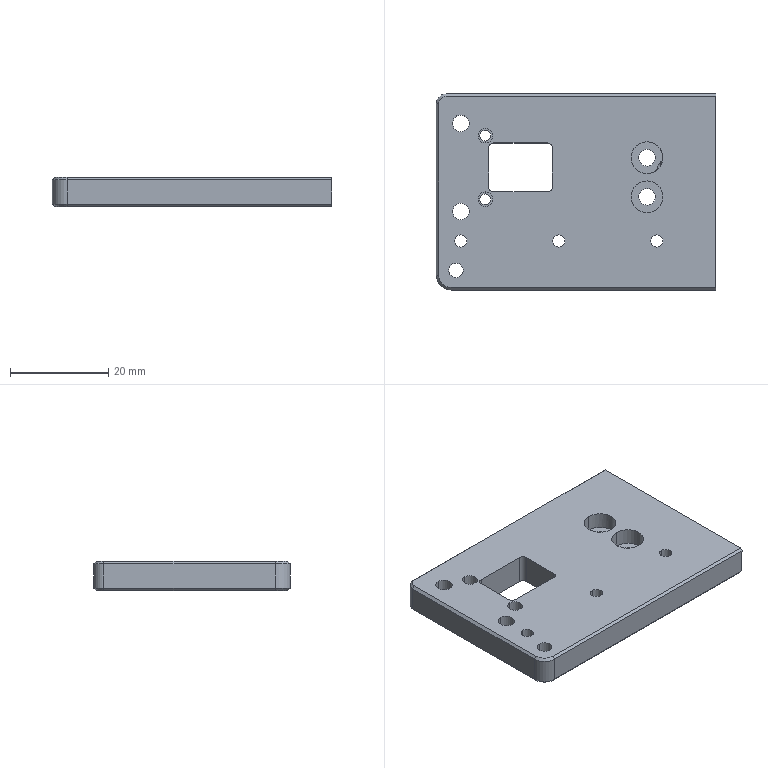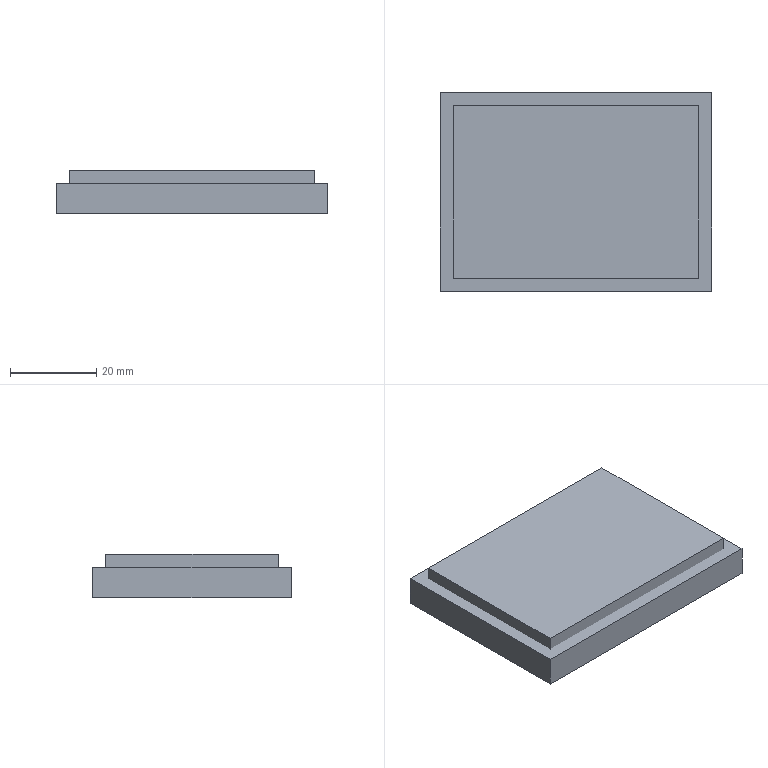CAM job | NX | 3+2 milling, drilling | part box 57 x 40 x 6 mm | stock box 63 x 46 x 10 mm
Tools:
number,name,description,diameter,corner_radius,flute_length,length,flutes
1,D50,Milling Tool-5 Parameters,50.0,0.0,50.0,75.0,2
7,D6A45,Milling Tool-5 Parameters,6.0,0.0,3.0,3.0,2
13,3.4ZT,Drilling Tool,3.4,0.0,35.0,50.0,2
11,2.5ZT,Drilling Tool,2.5,0.0,35.0,50.0,2
12,2.2ZT,Drilling Tool,2.2,0.0,35.0,50.0,2
10,D10,Milling Tool-5 Parameters,10.0,0.0,50.0,75.0,2
6,D6,Milling Tool-5 Parameters,6.0,0.0,50.0,75.0,2
4,D4,Milling Tool-5 Parameters,4.0,0.0,50.0,75.0,2
5,D2,Milling Tool-5 Parameters,2.0,0.0,50.0,75.0,2
Operations:
program,operation,operation_type,tool,method,geometry_group,spindle_rpm,surface_speed,feed_per_tooth,feed_cut,feed_plunge,cut_length_mm,path_length_mm,cut_time_min,machine_time_min
1-10-45-62毛胚-虎钳,FLOOR_WALL,VolumeBased25DMillingOperation,D50,METHOD,A,6500.0,1286.0,0.0962,1250.0,100.0,125.0,179.0,0.1,0.1054
1-10-45-62毛胚-虎钳,DRILLING_COPY_1,Operation,D6A45,METHOD,A,3000.0,56.0,0.0333,200.0,0.0,40.0,267.029,0.2,0.2227
1-10-45-62毛胚-虎钳,DRILLING_COPY_1_COPY_COPY_COPY_COPY,Operation,3.4ZT,METHOD,A,2000.0,21.0,0.0375,150.0,0.0,22.043,125.334,0.147,0.1573
1-10-45-62毛胚-虎钳,DRILLING_COPY_1_COPY_COPY_COPY_COPY_COPY,Operation,2.5ZT,METHOD,A,2000.0,15.0,0.0375,150.0,0.0,43.004,202.238,0.2867,0.3026
1-10-45-62毛胚-虎钳,DRILLING_COPY_1_COPY_COPY_COPY_COPY_COPY_COPY_COPY,Operation,2.2ZT,METHOD,A,2000.0,15.0,0.0375,150.0,0.0,21.322,118.986,0.1421,0.1519
1-10-45-62毛胚-虎钳,ZLEVEL_PROFILE,ZLevelMilling,D10,METHOD,A,7000.0,219.0,0.2143,3000.0,1000.0,2755.183,2818.183,0.9439,0.9502
1-10-45-62毛胚-虎钳,ZLEVEL_PROFILE_COPY,ZLevelMilling,D6,METHOD,A,7000.0,219.0,0.2143,3000.0,1000.0,371.774,434.774,0.1481,0.1544
1-10-45-62毛胚-虎钳,HOLE_MILLING,CylinderMilling,D4,METHOD,A,7000.0,131.0,0.1071,1500.0,100.0,227.914,361.714,0.1519,0.1653
1-10-45-62毛胚-虎钳,ZLEVEL_PROFILE_COPY_1,ZLevelMilling,D4,METHOD,A,7000.0,87.0,0.1071,1500.0,1000.0,289.284,660.942,0.2151,0.2523
1-10-45-62毛胚-虎钳,ZLEVEL_PROFILE_COPY_COPY_1_COPY_COPY_COPY_1,ZLevelMilling,D4,METHOD,A,7000.0,219.0,0.0714,1000.0,100.0,236.993,405.609,0.237,0.2539
1-10-45-62毛胚-虎钳,ZLEVEL_PROFILE_COPY_1_COPY,ZLevelMilling,D2,METHOD,A,7000.0,43.0,0.0786,1100.0,1000.0,593.553,1151.035,0.5477,0.6034
1-10-45-62毛胚-虎钳,HOLE_MILLING_COPY,CylinderMilling,D2,METHOD,A,7000.0,43.0,0.0786,1100.0,100.0,343.055,566.247,0.3119,0.3342
1-10-45-62毛胚-虎钳,ZLEVEL_PROFILE_COPY_1_COPY_COPY_COPY_COPY_2_COPY_COPY_1,ZLevelMilling,D6A45,METHOD,A,7000.0,131.0,0.0714,1000.0,1000.0,311.892,1359.408,0.3119,0.4166
1-10-45-62毛胚-虎钳,刀补5,CylinderMilling,D2,METHOD,A,7000.0,43.0,0.0607,850.0,100.0,66.487,289.679,0.0782,0.1005
2-10-45-62毛胚毛胚-虎钳,FLOOR_WALL_COPY,VolumeBased25DMillingOperation,D50,METHOD,B,6500.0,1286.0,0.0962,1250.0,100.0,476.0,1019.001,0.3808,0.4351
2-10-45-62毛胚毛胚-虎钳,DRILLING_COPY_1_COPY,Operation,D6A45,METHOD,B,3000.0,56.0,0.0333,200.0,0.0,9.7,90.944,0.0485,0.0566
2-10-45-62毛胚毛胚-虎钳,DRILLING_COPY_1_COPY_COPY,Operation,D6A45,METHOD,B,3000.0,56.0,0.0333,200.0,0.0,8.4,93.142,0.042,0.0505
2-10-45-62毛胚毛胚-虎钳,DRILLING_COPY_1_COPY_COPY_COPY_COPY_COPY_1,Operation,3.4ZT,METHOD,B,2000.0,21.0,0.0375,150.0,0.0,22.043,115.63,0.147,0.1563
2-10-45-62毛胚毛胚-虎钳,HOLE_MILLING_COPY_1,CylinderMilling,D4,METHOD,B,7000.0,131.0,0.1071,1500.0,100.0,227.914,371.714,0.1519,0.1663
2-10-45-62毛胚毛胚-虎钳,ZLEVEL_PROFILE_COPY_1_COPY_COPY_COPY_COPY_2_COPY_COPY_1_COPY,ZLevelMilling,D6A45,METHOD,B,7000.0,131.0,0.0714,1000.0,1000.0,302.579,1188.701,0.3026,0.3912
3-10-45-62毛胚毛胚-虎钳,DRILLING_COPY_1_COPY_1,Operation,D6A45,METHOD,C,3000.0,56.0,0.0333,200.0,0.0,23.0,140.485,0.115,0.1267
3-10-45-62毛胚毛胚-虎钳,DRILLING_COPY_1_COPY_COPY_COPY_COPY_COPY_COPY,Operation,2.5ZT,METHOD,C,2000.0,15.0,0.0375,150.0,0.0,70.406,235.296,0.4694,0.4859
3-10-45-62毛胚毛胚-虎钳,ZLEVEL_PROFILE_1,ZLevelMilling,D2,METHOD,C,7000.0,65.0,0.0786,1100.0,1000.0,499.272,641.853,0.4579,0.4721
3-10-45-62毛胚毛胚-虎钳,ZLEVEL_PROFILE_COPY_1_COPY_COPY_COPY_COPY_2_COPY_COPY_1_1_COPY_1,ZLevelMilling,D6A45,METHOD,C,7000.0,131.0,0.0714,1000.0,1000.0,21.182,360.298,0.0212,0.0551
3-10-45-62毛胚毛胚-虎钳,刀补5.,ZLevelMilling,D2,METHOD,C,7000.0,65.0,0.0786,1100.0,1000.0,80.286,227.427,0.0731,0.0879